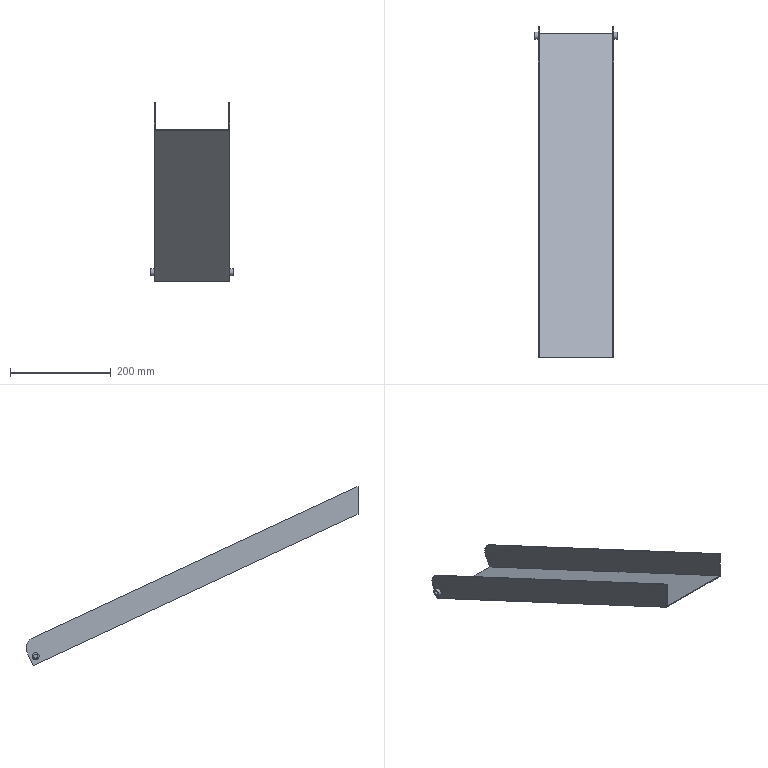Part | NX | features solid 2 | 1 solid | 20 faces | box 163.6 x 659.089 x 355.721 mm | volume 353429 mm3 | plane 14 | cylinder 6 | commonest cylinder face diameters 8 x2 14 x2 40 x2
STEP:
#1=CARTESIAN_POINT('',(230.,600.,-318.114));
#2=VERTEX_POINT('',#1);
#3=CARTESIAN_POINT('',(230.,600.,-262.945));
#4=VERTEX_POINT('',#3);
#5=CARTESIAN_POINT('',(230.,600.,-618.666));
#6=DIRECTION('',(0.,0.,1.));
#7=VECTOR('',#6,1000.);
#8=LINE('',#5,#7);
#9=EDGE_CURVE('',#2,#4,#8,.T.);
#10=ORIENTED_EDGE('',*,*,#9,.F.);
#11=CARTESIAN_POINT('',(230.,1244.536,-618.666));
#12=VERTEX_POINT('',#11);
#13=CARTESIAN_POINT('',(230.,1244.536,-618.666));
#14=DIRECTION('',(0.,-0.9063,0.4226));
#15=VECTOR('',#14,1000.);
#16=LINE('',#13,#15);
#17=EDGE_CURVE('',#12,#2,#16,.T.);
#18=ORIENTED_EDGE('',*,*,#17,.F.);
#19=CARTESIAN_POINT('',(230.,1257.215,-591.477));
#20=VERTEX_POINT('',#19);
#21=CARTESIAN_POINT('',(230.,1244.536,-618.666));
#22=DIRECTION('',(0.,0.4226,0.9063));
#23=VECTOR('',#22,1000.);
#24=LINE('',#21,#23);
#25=EDGE_CURVE('',#12,#20,#24,.T.);
#26=ORIENTED_EDGE('',*,*,#25,.T.);
#27=CARTESIAN_POINT('',(230.,1247.541,-564.898));
#28=VERTEX_POINT('',#27);
#29=CARTESIAN_POINT('',(230.,1239.089,-583.024));
#30=DIRECTION('',(-1.,0.,0.));
#31=DIRECTION('',(0.,-1.,0.));
#32=AXIS2_PLACEMENT_3D('',#29,#30,#31);
#33=CIRCLE('',#32,20.);
#34=EDGE_CURVE('',#28,#20,#33,.T.);
#35=ORIENTED_EDGE('',*,*,#34,.F.);
#36=CARTESIAN_POINT('',(230.,1247.541,-564.898));
#37=DIRECTION('',(0.,-0.9063,0.4226));
#38=VECTOR('',#37,1000.);
#39=LINE('',#36,#38);
#40=EDGE_CURVE('',#28,#4,#39,.T.);
#41=ORIENTED_EDGE('',*,*,#40,.T.);
#42=EDGE_LOOP('',(#10,#18,#26,#35,#41));
#43=FACE_BOUND('',#42,.T.);
#44=CARTESIAN_POINT('',(230.,1240.,-593.));
#45=VERTEX_POINT('',#44);
#46=CARTESIAN_POINT('',(230.,1240.,-600.));
#47=DIRECTION('',(1.,0.,0.));
#48=DIRECTION('',(0.,0.,1.));
#49=AXIS2_PLACEMENT_3D('',#46,#47,#48);
#50=CIRCLE('',#49,7.);
#51=EDGE_CURVE('',#45,#45,#50,.F.);
#52=ORIENTED_EDGE('',*,*,#51,.T.);
#53=EDGE_LOOP('',(#52));
#54=FACE_BOUND('',#53,.T.);
#55=CARTESIAN_POINT('',(230.,1244.536,-618.666));
#56=DIRECTION('',(1.,0.,0.));
#57=DIRECTION('',(0.,-0.9063,0.4226));
#58=AXIS2_PLACEMENT_3D('',#55,#56,#57);
#59=PLANE('',#58);
#60=ADVANCED_FACE('',(#43,#54),#59,.T.);
#61=CARTESIAN_POINT('',(82.,600.,-315.907));
#62=VERTEX_POINT('',#61);
#63=CARTESIAN_POINT('',(82.,1245.382,-616.853));
#64=VERTEX_POINT('',#63);
#65=CARTESIAN_POINT('',(82.,1245.382,-616.853));
#66=DIRECTION('',(0.,0.9063,-0.4226));
#67=VECTOR('',#66,1000.);
#68=LINE('',#65,#67);
#69=EDGE_CURVE('',#62,#64,#68,.T.);
#70=ORIENTED_EDGE('',*,*,#69,.F.);
#71=CARTESIAN_POINT('',(228.,600.,-315.907));
#72=VERTEX_POINT('',#71);
#73=CARTESIAN_POINT('',(230.,600.,-315.907));
#74=DIRECTION('',(1.,0.,0.));
#75=VECTOR('',#74,1000.);
#76=LINE('',#73,#75);
#77=EDGE_CURVE('',#62,#72,#76,.T.);
#78=ORIENTED_EDGE('',*,*,#77,.T.);
#79=CARTESIAN_POINT('',(228.,1245.382,-616.853));
#80=VERTEX_POINT('',#79);
#81=CARTESIAN_POINT('',(228.,1245.382,-616.853));
#82=DIRECTION('',(0.,0.9063,-0.4226));
#83=VECTOR('',#82,1000.);
#84=LINE('',#81,#83);
#85=EDGE_CURVE('',#72,#80,#84,.T.);
#86=ORIENTED_EDGE('',*,*,#85,.T.);
#87=CARTESIAN_POINT('',(230.,1245.382,-616.853));
#88=DIRECTION('',(1.,0.,0.));
#89=VECTOR('',#88,1000.);
#90=LINE('',#87,#89);
#91=EDGE_CURVE('',#80,#64,#90,.F.);
#92=ORIENTED_EDGE('',*,*,#91,.T.);
#93=EDGE_LOOP('',(#70,#78,#86,#92));
#94=FACE_BOUND('',#93,.T.);
#95=CARTESIAN_POINT('',(230.,1245.382,-616.853));
#96=DIRECTION('',(0.,-0.4226,-0.9063));
#97=DIRECTION('',(0.,0.9063,-0.4226));
#98=AXIS2_PLACEMENT_3D('',#95,#96,#97);
#99=PLANE('',#98);
#100=ADVANCED_FACE('',(#94),#99,.F.);
#101=CARTESIAN_POINT('',(82.,1257.215,-591.477));
#102=VERTEX_POINT('',#101);
#103=CARTESIAN_POINT('',(82.,1257.215,-591.477));
#104=DIRECTION('',(0.,-0.4226,-0.9063));
#105=VECTOR('',#104,1000.);
#106=LINE('',#103,#105);
#107=EDGE_CURVE('',#102,#64,#106,.T.);
#108=ORIENTED_EDGE('',*,*,#107,.T.);
#109=ORIENTED_EDGE('',*,*,#91,.F.);
#110=CARTESIAN_POINT('',(228.,1257.215,-591.477));
#111=VERTEX_POINT('',#110);
#112=CARTESIAN_POINT('',(228.,1257.215,-591.477));
#113=DIRECTION('',(0.,-0.4226,-0.9063));
#114=VECTOR('',#113,1000.);
#115=LINE('',#112,#114);
#116=EDGE_CURVE('',#111,#80,#115,.T.);
#117=ORIENTED_EDGE('',*,*,#116,.F.);
#118=CARTESIAN_POINT('',(228.,1257.215,-591.477));
#119=DIRECTION('',(1.,0.,0.));
#120=VECTOR('',#119,1000.);
#121=LINE('',#118,#120);
#122=EDGE_CURVE('',#111,#20,#121,.T.);
#123=ORIENTED_EDGE('',*,*,#122,.T.);
#124=ORIENTED_EDGE('',*,*,#25,.F.);
#125=CARTESIAN_POINT('',(80.,1244.536,-618.666));
#126=VERTEX_POINT('',#125);
#127=CARTESIAN_POINT('',(230.,1244.536,-618.666));
#128=DIRECTION('',(-1.,0.,0.));
#129=VECTOR('',#128,1000.);
#130=LINE('',#127,#129);
#131=EDGE_CURVE('',#12,#126,#130,.T.);
#132=ORIENTED_EDGE('',*,*,#131,.T.);
#133=CARTESIAN_POINT('',(80.,1257.215,-591.477));
#134=VERTEX_POINT('',#133);
#135=CARTESIAN_POINT('',(80.,1244.536,-618.666));
#136=DIRECTION('',(0.,0.4226,0.9063));
#137=VECTOR('',#136,1000.);
#138=LINE('',#135,#137);
#139=EDGE_CURVE('',#126,#134,#138,.T.);
#140=ORIENTED_EDGE('',*,*,#139,.T.);
#141=CARTESIAN_POINT('',(82.,1257.215,-591.477));
#142=DIRECTION('',(-1.,0.,0.));
#143=VECTOR('',#142,1000.);
#144=LINE('',#141,#143);
#145=EDGE_CURVE('',#102,#134,#144,.T.);
#146=ORIENTED_EDGE('',*,*,#145,.F.);
#147=EDGE_LOOP('',(#108,#109,#117,#123,#124,#132,#140,#146));
#148=FACE_BOUND('',#147,.T.);
#149=CARTESIAN_POINT('',(230.,1244.536,-618.666));
#150=DIRECTION('',(0.,-0.9063,0.4226));
#151=DIRECTION('',(-1.,0.,0.));
#152=AXIS2_PLACEMENT_3D('',#149,#150,#151);
#153=PLANE('',#152);
#154=ADVANCED_FACE('',(#148),#153,.F.);
#155=CARTESIAN_POINT('',(80.,600.,-262.945));
#156=VERTEX_POINT('',#155);
#157=CARTESIAN_POINT('',(80.,600.,-318.114));
#158=VERTEX_POINT('',#157);
#159=CARTESIAN_POINT('',(80.,600.,-618.666));
#160=DIRECTION('',(0.,0.,1.));
#161=VECTOR('',#160,1000.);
#162=LINE('',#159,#161);
#163=EDGE_CURVE('',#156,#158,#162,.F.);
#164=ORIENTED_EDGE('',*,*,#163,.F.);
#165=CARTESIAN_POINT('',(80.,1247.541,-564.898));
#166=VERTEX_POINT('',#165);
#167=CARTESIAN_POINT('',(80.,1247.541,-564.898));
#168=DIRECTION('',(0.,-0.9063,0.4226));
#169=VECTOR('',#168,1000.);
#170=LINE('',#167,#169);
#171=EDGE_CURVE('',#166,#156,#170,.T.);
#172=ORIENTED_EDGE('',*,*,#171,.F.);
#173=CARTESIAN_POINT('',(80.,1239.089,-583.024));
#174=DIRECTION('',(-1.,0.,0.));
#175=DIRECTION('',(0.,-1.,0.));
#176=AXIS2_PLACEMENT_3D('',#173,#174,#175);
#177=CIRCLE('',#176,20.);
#178=EDGE_CURVE('',#166,#134,#177,.T.);
#179=ORIENTED_EDGE('',*,*,#178,.T.);
#180=ORIENTED_EDGE('',*,*,#139,.F.);
#181=CARTESIAN_POINT('',(80.,1244.536,-618.666));
#182=DIRECTION('',(0.,-0.9063,0.4226));
#183=VECTOR('',#182,1000.);
#184=LINE('',#181,#183);
#185=EDGE_CURVE('',#126,#158,#184,.T.);
#186=ORIENTED_EDGE('',*,*,#185,.T.);
#187=EDGE_LOOP('',(#164,#172,#179,#180,#186));
#188=FACE_BOUND('',#187,.T.);
#189=CARTESIAN_POINT('',(80.,1240.,-593.));
#190=VERTEX_POINT('',#189);
#191=CARTESIAN_POINT('',(80.,1240.,-600.));
#192=DIRECTION('',(1.,0.,0.));
#193=DIRECTION('',(0.,0.,1.));
#194=AXIS2_PLACEMENT_3D('',#191,#192,#193);
#195=CIRCLE('',#194,7.);
#196=EDGE_CURVE('',#190,#190,#195,.F.);
#197=ORIENTED_EDGE('',*,*,#196,.F.);
#198=EDGE_LOOP('',(#197));
#199=FACE_BOUND('',#198,.T.);
#200=CARTESIAN_POINT('',(80.,1244.536,-618.666));
#201=DIRECTION('',(1.,0.,0.));
#202=DIRECTION('',(0.,-0.9063,0.4226));
#203=AXIS2_PLACEMENT_3D('',#200,#201,#202);
#204=PLANE('',#203);
#205=ADVANCED_FACE('',(#188,#199),#204,.F.);
#206=CARTESIAN_POINT('',(230.,600.,-318.114));
#207=DIRECTION('',(1.,0.,0.));
#208=VECTOR('',#207,1000.);
#209=LINE('',#206,#208);
#210=EDGE_CURVE('',#158,#2,#209,.T.);
#211=ORIENTED_EDGE('',*,*,#210,.F.);
#212=ORIENTED_EDGE('',*,*,#185,.F.);
#213=ORIENTED_EDGE('',*,*,#131,.F.);
#214=ORIENTED_EDGE('',*,*,#17,.T.);
#215=EDGE_LOOP('',(#211,#212,#213,#214));
#216=FACE_BOUND('',#215,.T.);
#217=CARTESIAN_POINT('',(230.,1244.536,-618.666));
#218=DIRECTION('',(0.,-0.4226,-0.9063));
#219=DIRECTION('',(0.,0.9063,-0.4226));
#220=AXIS2_PLACEMENT_3D('',#217,#218,#219);
#221=PLANE('',#220);
#222=ADVANCED_FACE('',(#216),#221,.T.);
#223=CARTESIAN_POINT('',(228.,600.,-262.945));
#224=VERTEX_POINT('',#223);
#225=CARTESIAN_POINT('',(228.,600.,-502.116));
#226=DIRECTION('',(0.,0.,-1.));
#227=VECTOR('',#226,1000.);
#228=LINE('',#225,#227);
#229=EDGE_CURVE('',#224,#72,#228,.T.);
#230=ORIENTED_EDGE('',*,*,#229,.F.);
#231=CARTESIAN_POINT('',(228.,1247.541,-564.898));
#232=VERTEX_POINT('',#231);
#233=CARTESIAN_POINT('',(228.,1247.541,-564.898));
#234=DIRECTION('',(0.,-0.9063,0.4226));
#235=VECTOR('',#234,1000.);
#236=LINE('',#233,#235);
#237=EDGE_CURVE('',#232,#224,#236,.T.);
#238=ORIENTED_EDGE('',*,*,#237,.F.);
#239=CARTESIAN_POINT('',(228.,1239.089,-583.024));
#240=DIRECTION('',(-1.,0.,0.));
#241=DIRECTION('',(0.,-1.,0.));
#242=AXIS2_PLACEMENT_3D('',#239,#240,#241);
#243=CIRCLE('',#242,20.);
#244=EDGE_CURVE('',#232,#111,#243,.T.);
#245=ORIENTED_EDGE('',*,*,#244,.T.);
#246=ORIENTED_EDGE('',*,*,#116,.T.);
#247=ORIENTED_EDGE('',*,*,#85,.F.);
#248=EDGE_LOOP('',(#230,#238,#245,#246,#247));
#249=FACE_BOUND('',#248,.T.);
#250=CARTESIAN_POINT('',(228.,1089.243,-502.116));
#251=DIRECTION('',(-1.,0.,0.));
#252=DIRECTION('',(0.,0.,-1.));
#253=AXIS2_PLACEMENT_3D('',#250,#251,#252);
#254=PLANE('',#253);
#255=ADVANCED_FACE('',(#249),#254,.T.);
#256=CARTESIAN_POINT('',(228.,600.,-262.945));
#257=DIRECTION('',(-1.,0.,0.));
#258=VECTOR('',#257,1000.);
#259=LINE('',#256,#258);
#260=EDGE_CURVE('',#4,#224,#259,.T.);
#261=ORIENTED_EDGE('',*,*,#260,.F.);
#262=ORIENTED_EDGE('',*,*,#40,.F.);
#263=CARTESIAN_POINT('',(228.,1247.541,-564.898));
#264=DIRECTION('',(1.,0.,0.));
#265=VECTOR('',#264,1000.);
#266=LINE('',#263,#265);
#267=EDGE_CURVE('',#232,#28,#266,.T.);
#268=ORIENTED_EDGE('',*,*,#267,.F.);
#269=ORIENTED_EDGE('',*,*,#237,.T.);
#270=EDGE_LOOP('',(#261,#262,#268,#269));
#271=FACE_BOUND('',#270,.T.);
#272=CARTESIAN_POINT('',(228.,1247.541,-564.898));
#273=DIRECTION('',(0.,0.4226,0.9063));
#274=DIRECTION('',(0.,-0.9063,0.4226));
#275=AXIS2_PLACEMENT_3D('',#272,#273,#274);
#276=PLANE('',#275);
#277=ADVANCED_FACE('',(#271),#276,.T.);
#278=ORIENTED_EDGE('',*,*,#34,.T.);
#279=ORIENTED_EDGE('',*,*,#122,.F.);
#280=ORIENTED_EDGE('',*,*,#244,.F.);
#281=ORIENTED_EDGE('',*,*,#267,.T.);
#282=EDGE_LOOP('',(#278,#279,#280,#281));
#283=FACE_BOUND('',#282,.T.);
#284=CARTESIAN_POINT('',(228.,1239.089,-583.024));
#285=DIRECTION('',(1.,0.,0.));
#286=DIRECTION('',(0.,0.,1.));
#287=AXIS2_PLACEMENT_3D('',#284,#285,#286);
#288=CYLINDRICAL_SURFACE('',#287,20.);
#289=ADVANCED_FACE('',(#283),#288,.T.);
#290=CARTESIAN_POINT('',(82.,1247.541,-564.898));
#291=VERTEX_POINT('',#290);
#292=CARTESIAN_POINT('',(82.,600.,-262.945));
#293=VERTEX_POINT('',#292);
#294=CARTESIAN_POINT('',(82.,1247.541,-564.898));
#295=DIRECTION('',(0.,-0.9063,0.4226));
#296=VECTOR('',#295,1000.);
#297=LINE('',#294,#296);
#298=EDGE_CURVE('',#291,#293,#297,.T.);
#299=ORIENTED_EDGE('',*,*,#298,.T.);
#300=CARTESIAN_POINT('',(82.,600.,-502.116));
#301=DIRECTION('',(0.,0.,-1.));
#302=VECTOR('',#301,1000.);
#303=LINE('',#300,#302);
#304=EDGE_CURVE('',#293,#62,#303,.T.);
#305=ORIENTED_EDGE('',*,*,#304,.T.);
#306=ORIENTED_EDGE('',*,*,#69,.T.);
#307=ORIENTED_EDGE('',*,*,#107,.F.);
#308=CARTESIAN_POINT('',(82.,1239.089,-583.024));
#309=DIRECTION('',(-1.,0.,0.));
#310=DIRECTION('',(0.,-1.,0.));
#311=AXIS2_PLACEMENT_3D('',#308,#309,#310);
#312=CIRCLE('',#311,20.);
#313=EDGE_CURVE('',#291,#102,#312,.T.);
#314=ORIENTED_EDGE('',*,*,#313,.F.);
#315=EDGE_LOOP('',(#299,#305,#306,#307,#314));
#316=FACE_BOUND('',#315,.T.);
#317=CARTESIAN_POINT('',(82.,1089.243,-502.116));
#318=DIRECTION('',(-1.,0.,0.));
#319=DIRECTION('',(0.,0.,-1.));
#320=AXIS2_PLACEMENT_3D('',#317,#318,#319);
#321=PLANE('',#320);
#322=ADVANCED_FACE('',(#316),#321,.F.);
#323=ORIENTED_EDGE('',*,*,#171,.T.);
#324=CARTESIAN_POINT('',(82.,600.,-262.945));
#325=DIRECTION('',(1.,0.,0.));
#326=VECTOR('',#325,1000.);
#327=LINE('',#324,#326);
#328=EDGE_CURVE('',#156,#293,#327,.T.);
#329=ORIENTED_EDGE('',*,*,#328,.T.);
#330=ORIENTED_EDGE('',*,*,#298,.F.);
#331=CARTESIAN_POINT('',(82.,1247.541,-564.898));
#332=DIRECTION('',(-1.,0.,0.));
#333=VECTOR('',#332,1000.);
#334=LINE('',#331,#333);
#335=EDGE_CURVE('',#291,#166,#334,.T.);
#336=ORIENTED_EDGE('',*,*,#335,.T.);
#337=EDGE_LOOP('',(#323,#329,#330,#336));
#338=FACE_BOUND('',#337,.T.);
#339=CARTESIAN_POINT('',(82.,1247.541,-564.898));
#340=DIRECTION('',(0.,-0.4226,-0.9063));
#341=DIRECTION('',(0.,0.9063,-0.4226));
#342=AXIS2_PLACEMENT_3D('',#339,#340,#341);
#343=PLANE('',#342);
#344=ADVANCED_FACE('',(#338),#343,.F.);
#345=ORIENTED_EDGE('',*,*,#178,.F.);
#346=ORIENTED_EDGE('',*,*,#335,.F.);
#347=ORIENTED_EDGE('',*,*,#313,.T.);
#348=ORIENTED_EDGE('',*,*,#145,.T.);
#349=EDGE_LOOP('',(#345,#346,#347,#348));
#350=FACE_BOUND('',#349,.T.);
#351=CARTESIAN_POINT('',(82.,1239.089,-583.024));
#352=DIRECTION('',(-1.,0.,0.));
#353=DIRECTION('',(0.,0.,-1.));
#354=AXIS2_PLACEMENT_3D('',#351,#352,#353);
#355=CYLINDRICAL_SURFACE('',#354,20.);
#356=ADVANCED_FACE('',(#350),#355,.T.);
#357=CARTESIAN_POINT('',(73.2,1240.,-607.));
#358=VERTEX_POINT('',#357);
#359=CARTESIAN_POINT('',(73.2,1240.,-600.));
#360=DIRECTION('',(-1.,0.,0.));
#361=DIRECTION('',(0.,0.,-1.));
#362=AXIS2_PLACEMENT_3D('',#359,#360,#361);
#363=CIRCLE('',#362,7.);
#364=EDGE_CURVE('',#358,#358,#363,.T.);
#365=ORIENTED_EDGE('',*,*,#364,.T.);
#366=EDGE_LOOP('',(#365));
#367=FACE_BOUND('',#366,.T.);
#368=CARTESIAN_POINT('',(73.2,1236.,-600.));
#369=VERTEX_POINT('',#368);
#370=CARTESIAN_POINT('',(73.2,1240.,-600.));
#371=DIRECTION('',(-1.,0.,0.));
#372=DIRECTION('',(0.,-1.,0.));
#373=AXIS2_PLACEMENT_3D('',#370,#371,#372);
#374=CIRCLE('',#373,4.);
#375=EDGE_CURVE('',#369,#369,#374,.T.);
#376=ORIENTED_EDGE('',*,*,#375,.F.);
#377=EDGE_LOOP('',(#376));
#378=FACE_BOUND('',#377,.T.);
#379=CARTESIAN_POINT('',(73.2,1240.,-600.));
#380=DIRECTION('',(1.,0.,0.));
#381=DIRECTION('',(0.,0.,1.));
#382=AXIS2_PLACEMENT_3D('',#379,#380,#381);
#383=PLANE('',#382);
#384=ADVANCED_FACE('',(#367,#378),#383,.F.);
#385=ORIENTED_EDGE('',*,*,#364,.F.);
#386=EDGE_LOOP('',(#385));
#387=FACE_BOUND('',#386,.T.);
#388=ORIENTED_EDGE('',*,*,#196,.T.);
#389=EDGE_LOOP('',(#388));
#390=FACE_BOUND('',#389,.T.);
#391=CARTESIAN_POINT('',(80.,1240.,-600.));
#392=DIRECTION('',(-1.,0.,0.));
#393=DIRECTION('',(0.,0.,-1.));
#394=AXIS2_PLACEMENT_3D('',#391,#392,#393);
#395=CYLINDRICAL_SURFACE('',#394,7.);
#396=ADVANCED_FACE('',(#387,#390),#395,.T.);
#397=ORIENTED_EDGE('',*,*,#375,.T.);
#398=EDGE_LOOP('',(#397));
#399=FACE_BOUND('',#398,.T.);
#400=CARTESIAN_POINT('',(80.,1236.,-600.));
#401=VERTEX_POINT('',#400);
#402=CARTESIAN_POINT('',(80.,1240.,-600.));
#403=DIRECTION('',(-1.,0.,0.));
#404=DIRECTION('',(0.,-1.,0.));
#405=AXIS2_PLACEMENT_3D('',#402,#403,#404);
#406=CIRCLE('',#405,4.);
#407=EDGE_CURVE('',#401,#401,#406,.T.);
#408=ORIENTED_EDGE('',*,*,#407,.F.);
#409=EDGE_LOOP('',(#408));
#410=FACE_BOUND('',#409,.T.);
#411=CARTESIAN_POINT('',(80.,1240.,-600.));
#412=DIRECTION('',(-1.,0.,0.));
#413=DIRECTION('',(0.,0.,-1.));
#414=AXIS2_PLACEMENT_3D('',#411,#412,#413);
#415=CYLINDRICAL_SURFACE('',#414,4.);
#416=ADVANCED_FACE('',(#399,#410),#415,.F.);
#417=ORIENTED_EDGE('',*,*,#407,.T.);
#418=EDGE_LOOP('',(#417));
#419=FACE_BOUND('',#418,.T.);
#420=CARTESIAN_POINT('',(80.,1244.536,-618.666));
#421=DIRECTION('',(1.,0.,0.));
#422=DIRECTION('',(0.,-0.9063,0.4226));
#423=AXIS2_PLACEMENT_3D('',#420,#421,#422);
#424=PLANE('',#423);
#425=ADVANCED_FACE('',(#419),#424,.F.);
#426=CARTESIAN_POINT('',(236.8,1240.,-593.));
#427=VERTEX_POINT('',#426);
#428=CARTESIAN_POINT('',(236.8,1240.,-600.));
#429=DIRECTION('',(1.,0.,0.));
#430=DIRECTION('',(0.,0.,1.));
#431=AXIS2_PLACEMENT_3D('',#428,#429,#430);
#432=CIRCLE('',#431,7.);
#433=EDGE_CURVE('',#427,#427,#432,.F.);
#434=ORIENTED_EDGE('',*,*,#433,.F.);
#435=EDGE_LOOP('',(#434));
#436=FACE_BOUND('',#435,.T.);
#437=CARTESIAN_POINT('',(236.8,1236.,-600.));
#438=VERTEX_POINT('',#437);
#439=CARTESIAN_POINT('',(236.8,1240.,-600.));
#440=DIRECTION('',(-1.,0.,0.));
#441=DIRECTION('',(0.,-1.,0.));
#442=AXIS2_PLACEMENT_3D('',#439,#440,#441);
#443=CIRCLE('',#442,4.);
#444=EDGE_CURVE('',#438,#438,#443,.T.);
#445=ORIENTED_EDGE('',*,*,#444,.T.);
#446=EDGE_LOOP('',(#445));
#447=FACE_BOUND('',#446,.T.);
#448=CARTESIAN_POINT('',(236.8,1240.,-600.));
#449=DIRECTION('',(1.,0.,0.));
#450=DIRECTION('',(0.,0.,1.));
#451=AXIS2_PLACEMENT_3D('',#448,#449,#450);
#452=PLANE('',#451);
#453=ADVANCED_FACE('',(#436,#447),#452,.T.);
#454=ORIENTED_EDGE('',*,*,#433,.T.);
#455=EDGE_LOOP('',(#454));
#456=FACE_BOUND('',#455,.T.);
#457=ORIENTED_EDGE('',*,*,#51,.F.);
#458=EDGE_LOOP('',(#457));
#459=FACE_BOUND('',#458,.T.);
#460=CARTESIAN_POINT('',(230.,1240.,-600.));
#461=DIRECTION('',(1.,0.,0.));
#462=DIRECTION('',(0.,0.,1.));
#463=AXIS2_PLACEMENT_3D('',#460,#461,#462);
#464=CYLINDRICAL_SURFACE('',#463,7.);
#465=ADVANCED_FACE('',(#456,#459),#464,.T.);
#466=ORIENTED_EDGE('',*,*,#444,.F.);
#467=EDGE_LOOP('',(#466));
#468=FACE_BOUND('',#467,.T.);
#469=CARTESIAN_POINT('',(230.,1240.,-596.));
#470=VERTEX_POINT('',#469);
#471=CARTESIAN_POINT('',(230.,1240.,-600.));
#472=DIRECTION('',(1.,0.,0.));
#473=DIRECTION('',(0.,0.,1.));
#474=AXIS2_PLACEMENT_3D('',#471,#472,#473);
#475=CIRCLE('',#474,4.);
#476=EDGE_CURVE('',#470,#470,#475,.F.);
#477=ORIENTED_EDGE('',*,*,#476,.T.);
#478=EDGE_LOOP('',(#477));
#479=FACE_BOUND('',#478,.T.);
#480=CARTESIAN_POINT('',(230.,1240.,-600.));
#481=DIRECTION('',(1.,0.,0.));
#482=DIRECTION('',(0.,0.,1.));
#483=AXIS2_PLACEMENT_3D('',#480,#481,#482);
#484=CYLINDRICAL_SURFACE('',#483,4.);
#485=ADVANCED_FACE('',(#468,#479),#484,.F.);
#486=ORIENTED_EDGE('',*,*,#476,.F.);
#487=EDGE_LOOP('',(#486));
#488=FACE_BOUND('',#487,.T.);
#489=CARTESIAN_POINT('',(230.,1244.536,-618.666));
#490=DIRECTION('',(1.,0.,0.));
#491=DIRECTION('',(0.,-0.9063,0.4226));
#492=AXIS2_PLACEMENT_3D('',#489,#490,#491);
#493=PLANE('',#492);
#494=ADVANCED_FACE('',(#488),#493,.T.);
#495=ORIENTED_EDGE('',*,*,#9,.T.);
#496=ORIENTED_EDGE('',*,*,#260,.T.);
#497=ORIENTED_EDGE('',*,*,#229,.T.);
#498=ORIENTED_EDGE('',*,*,#77,.F.);
#499=ORIENTED_EDGE('',*,*,#304,.F.);
#500=ORIENTED_EDGE('',*,*,#328,.F.);
#501=ORIENTED_EDGE('',*,*,#163,.T.);
#502=ORIENTED_EDGE('',*,*,#210,.T.);
#503=EDGE_LOOP('',(#495,#496,#497,#498,#499,#500,#501,#502));
#504=FACE_BOUND('',#503,.T.);
#505=CARTESIAN_POINT('',(0.,600.,-310.));
#506=DIRECTION('',(0.,1.,0.));
#507=DIRECTION('',(0.,0.,1.));
#508=AXIS2_PLACEMENT_3D('',#505,#506,#507);
#509=PLANE('',#508);
#510=ADVANCED_FACE('',(#504),#509,.F.);
#511=CLOSED_SHELL('',(#60,#100,#154,#205,#222,#255,#277,#289,#322,#344,#356,#384,#396,#416,#425,#453,#465,#485,#494,#510));
#512=MANIFOLD_SOLID_BREP('',#511);
#513=(LENGTH_UNIT()NAMED_UNIT(*)SI_UNIT(.MILLI.,.METRE.));
#514=UNCERTAINTY_MEASURE_WITH_UNIT(LENGTH_MEASURE(0.00001),#513,'','');
#515=(NAMED_UNIT(*)PLANE_ANGLE_UNIT()SI_UNIT($,.RADIAN.));
#516=(NAMED_UNIT(*)SI_UNIT($,.STERADIAN.)SOLID_ANGLE_UNIT());
#517=(GEOMETRIC_REPRESENTATION_CONTEXT(3)GLOBAL_UNCERTAINTY_ASSIGNED_CONTEXT((#514))GLOBAL_UNIT_ASSIGNED_CONTEXT((#513,#515,#516))REPRESENTATION_CONTEXT('',''));
#518=ADVANCED_BREP_SHAPE_REPRESENTATION('',(#512),#517);